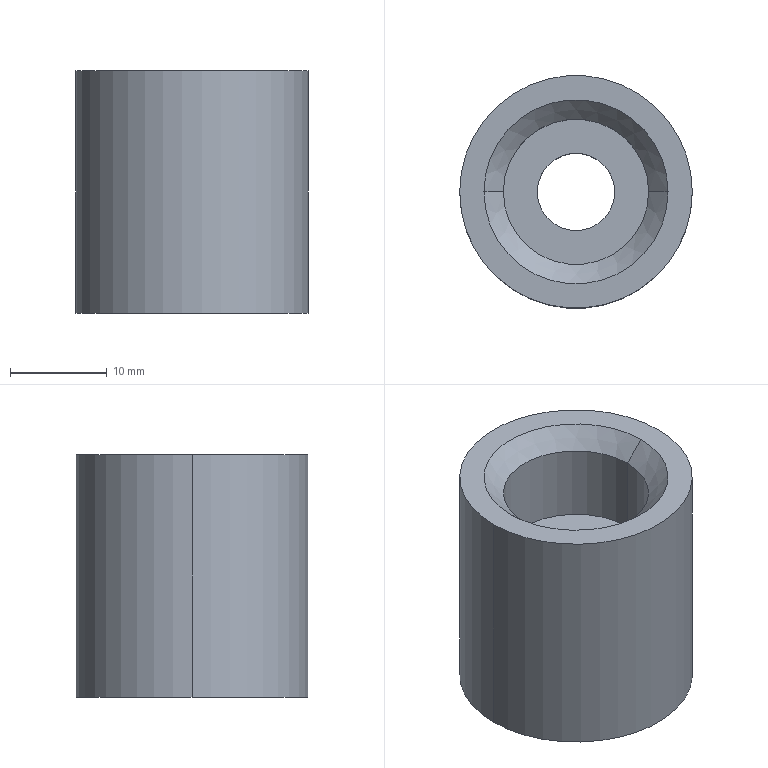Part | STEP file | Elastic block | 1 solid | 13 faces | box 24 x 24 x 25 mm | volume 8627 mm3 | cylinder 6 | cone 4 | plane 3 | commonest cylinder face diameters 8 x2 15 x2 24 x2
STEP:
#1=CARTESIAN_POINT('',(-12.,0.,25.));
#2=VERTEX_POINT('',#1);
#3=CARTESIAN_POINT('',(12.,0.,25.));
#4=VERTEX_POINT('',#3);
#5=CARTESIAN_POINT('',(0.,0.,25.));
#6=DIRECTION('',(0.,0.,-1.));
#7=DIRECTION('',(-1.,0.,0.));
#8=AXIS2_PLACEMENT_3D('',#5,#6,#7);
#9=CIRCLE('',#8,12.);
#10=EDGE_CURVE('',#2,#4,#9,.T.);
#11=ORIENTED_EDGE('',*,*,#10,.T.);
#12=CARTESIAN_POINT('',(12.,0.,0.));
#13=VERTEX_POINT('',#12);
#14=CARTESIAN_POINT('',(12.,0.,25.));
#15=DIRECTION('',(0.,0.,-1.));
#16=VECTOR('',#15,1000.);
#17=LINE('',#14,#16);
#18=EDGE_CURVE('',#4,#13,#17,.T.);
#19=ORIENTED_EDGE('',*,*,#18,.T.);
#20=CARTESIAN_POINT('',(-12.,0.,0.));
#21=VERTEX_POINT('',#20);
#22=CARTESIAN_POINT('',(0.,0.,0.));
#23=DIRECTION('',(0.,0.,1.));
#24=DIRECTION('',(-1.,0.,0.));
#25=AXIS2_PLACEMENT_3D('',#22,#23,#24);
#26=CIRCLE('',#25,12.);
#27=EDGE_CURVE('',#13,#21,#26,.T.);
#28=ORIENTED_EDGE('',*,*,#27,.T.);
#29=CARTESIAN_POINT('',(-12.,0.,25.));
#30=DIRECTION('',(0.,0.,-1.));
#31=VECTOR('',#30,1000.);
#32=LINE('',#29,#31);
#33=EDGE_CURVE('',#2,#21,#32,.T.);
#34=ORIENTED_EDGE('',*,*,#33,.F.);
#35=EDGE_LOOP('',(#11,#19,#28,#34));
#36=FACE_OUTER_BOUND('',#35,.T.);
#37=CARTESIAN_POINT('',(0.,0.,25.));
#38=DIRECTION('',(0.,0.,-1.));
#39=DIRECTION('',(-1.,0.,0.));
#40=AXIS2_PLACEMENT_3D('',#37,#38,#39);
#41=CYLINDRICAL_SURFACE('',#40,12.);
#42=ADVANCED_FACE('',(#36),#41,.T.);
#43=CARTESIAN_POINT('',(4.,0.,2.));
#44=VERTEX_POINT('',#43);
#45=CARTESIAN_POINT('',(-4.,0.,2.));
#46=VERTEX_POINT('',#45);
#47=CARTESIAN_POINT('',(0.,0.,2.));
#48=DIRECTION('',(0.,0.,-1.));
#49=DIRECTION('',(-1.,0.,0.));
#50=AXIS2_PLACEMENT_3D('',#47,#48,#49);
#51=CIRCLE('',#50,4.);
#52=EDGE_CURVE('',#44,#46,#51,.T.);
#53=ORIENTED_EDGE('',*,*,#52,.F.);
#54=CARTESIAN_POINT('',(6.,0.,0.));
#55=VERTEX_POINT('',#54);
#56=CARTESIAN_POINT('',(6.,0.,0.));
#57=DIRECTION('',(0.7071,0.,-0.7071));
#58=VECTOR('',#57,1000.);
#59=LINE('',#56,#58);
#60=EDGE_CURVE('',#44,#55,#59,.T.);
#61=ORIENTED_EDGE('',*,*,#60,.T.);
#62=CARTESIAN_POINT('',(-6.,0.,0.));
#63=VERTEX_POINT('',#62);
#64=CARTESIAN_POINT('',(0.,0.,0.));
#65=DIRECTION('',(0.,0.,-1.));
#66=DIRECTION('',(-1.,0.,0.));
#67=AXIS2_PLACEMENT_3D('',#64,#65,#66);
#68=CIRCLE('',#67,6.);
#69=EDGE_CURVE('',#55,#63,#68,.T.);
#70=ORIENTED_EDGE('',*,*,#69,.T.);
#71=CARTESIAN_POINT('',(-6.,0.,0.));
#72=DIRECTION('',(-0.7071,0.,-0.7071));
#73=VECTOR('',#72,1000.);
#74=LINE('',#71,#73);
#75=EDGE_CURVE('',#46,#63,#74,.T.);
#76=ORIENTED_EDGE('',*,*,#75,.F.);
#77=EDGE_LOOP('',(#53,#61,#70,#76));
#78=FACE_OUTER_BOUND('',#77,.T.);
#79=CARTESIAN_POINT('',(0.,0.,0.));
#80=DIRECTION('',(0.,0.,-1.));
#81=DIRECTION('',(-1.,0.,0.));
#82=AXIS2_PLACEMENT_3D('',#79,#80,#81);
#83=CONICAL_SURFACE('',#82,6.,0.7854);
#84=ADVANCED_FACE('',(#78),#83,.F.);
#85=CARTESIAN_POINT('',(-7.5,0.,23.));
#86=VERTEX_POINT('',#85);
#87=CARTESIAN_POINT('',(7.5,0.,23.));
#88=VERTEX_POINT('',#87);
#89=CARTESIAN_POINT('',(0.,0.,23.));
#90=DIRECTION('',(0.,0.,1.));
#91=DIRECTION('',(1.,0.,0.));
#92=AXIS2_PLACEMENT_3D('',#89,#90,#91);
#93=CIRCLE('',#92,7.5);
#94=EDGE_CURVE('',#86,#88,#93,.T.);
#95=ORIENTED_EDGE('',*,*,#94,.F.);
#96=CARTESIAN_POINT('',(-9.5,0.,25.));
#97=VERTEX_POINT('',#96);
#98=CARTESIAN_POINT('',(-9.5,0.,25.));
#99=DIRECTION('',(-0.7071,0.,0.7071));
#100=VECTOR('',#99,1000.);
#101=LINE('',#98,#100);
#102=EDGE_CURVE('',#86,#97,#101,.T.);
#103=ORIENTED_EDGE('',*,*,#102,.T.);
#104=CARTESIAN_POINT('',(9.5,0.,25.));
#105=VERTEX_POINT('',#104);
#106=CARTESIAN_POINT('',(0.,0.,25.));
#107=DIRECTION('',(0.,0.,-1.));
#108=DIRECTION('',(1.,0.,0.));
#109=AXIS2_PLACEMENT_3D('',#106,#107,#108);
#110=CIRCLE('',#109,9.5);
#111=EDGE_CURVE('',#105,#97,#110,.T.);
#112=ORIENTED_EDGE('',*,*,#111,.F.);
#113=CARTESIAN_POINT('',(9.5,0.,25.));
#114=DIRECTION('',(0.7071,0.,0.7071));
#115=VECTOR('',#114,1000.);
#116=LINE('',#113,#115);
#117=EDGE_CURVE('',#88,#105,#116,.T.);
#118=ORIENTED_EDGE('',*,*,#117,.F.);
#119=EDGE_LOOP('',(#95,#103,#112,#118));
#120=FACE_OUTER_BOUND('',#119,.T.);
#121=CARTESIAN_POINT('',(0.,0.,25.));
#122=DIRECTION('',(0.,0.,1.));
#123=DIRECTION('',(1.,0.,0.));
#124=AXIS2_PLACEMENT_3D('',#121,#122,#123);
#125=CONICAL_SURFACE('',#124,9.5,0.7854);
#126=ADVANCED_FACE('',(#120),#125,.F.);
#127=CARTESIAN_POINT('',(4.,0.,15.));
#128=VERTEX_POINT('',#127);
#129=CARTESIAN_POINT('',(-4.,0.,15.));
#130=VERTEX_POINT('',#129);
#131=CARTESIAN_POINT('',(0.,0.,15.));
#132=DIRECTION('',(0.,0.,-1.));
#133=DIRECTION('',(-1.,0.,0.));
#134=AXIS2_PLACEMENT_3D('',#131,#132,#133);
#135=CIRCLE('',#134,4.);
#136=EDGE_CURVE('',#128,#130,#135,.T.);
#137=ORIENTED_EDGE('',*,*,#136,.F.);
#138=CARTESIAN_POINT('',(4.,0.,25.));
#139=DIRECTION('',(0.,0.,-1.));
#140=VECTOR('',#139,1000.);
#141=LINE('',#138,#140);
#142=EDGE_CURVE('',#128,#44,#141,.T.);
#143=ORIENTED_EDGE('',*,*,#142,.T.);
#144=ORIENTED_EDGE('',*,*,#52,.T.);
#145=CARTESIAN_POINT('',(-4.,0.,25.));
#146=DIRECTION('',(0.,0.,-1.));
#147=VECTOR('',#146,1000.);
#148=LINE('',#145,#147);
#149=EDGE_CURVE('',#130,#46,#148,.T.);
#150=ORIENTED_EDGE('',*,*,#149,.F.);
#151=EDGE_LOOP('',(#137,#143,#144,#150));
#152=FACE_OUTER_BOUND('',#151,.T.);
#153=CARTESIAN_POINT('',(0.,0.,25.));
#154=DIRECTION('',(0.,0.,-1.));
#155=DIRECTION('',(-1.,0.,0.));
#156=AXIS2_PLACEMENT_3D('',#153,#154,#155);
#157=CYLINDRICAL_SURFACE('',#156,4.);
#158=ADVANCED_FACE('',(#152),#157,.F.);
#159=CARTESIAN_POINT('',(-7.5,0.,15.));
#160=VERTEX_POINT('',#159);
#161=CARTESIAN_POINT('',(7.5,0.,15.));
#162=VERTEX_POINT('',#161);
#163=CARTESIAN_POINT('',(0.,0.,15.));
#164=DIRECTION('',(0.,0.,1.));
#165=DIRECTION('',(1.,0.,0.));
#166=AXIS2_PLACEMENT_3D('',#163,#164,#165);
#167=CIRCLE('',#166,7.5);
#168=EDGE_CURVE('',#160,#162,#167,.T.);
#169=ORIENTED_EDGE('',*,*,#168,.F.);
#170=CARTESIAN_POINT('',(-7.5,0.,15.));
#171=DIRECTION('',(0.,0.,1.));
#172=VECTOR('',#171,1000.);
#173=LINE('',#170,#172);
#174=EDGE_CURVE('',#160,#86,#173,.T.);
#175=ORIENTED_EDGE('',*,*,#174,.T.);
#176=ORIENTED_EDGE('',*,*,#94,.T.);
#177=CARTESIAN_POINT('',(7.5,0.,15.));
#178=DIRECTION('',(0.,0.,1.));
#179=VECTOR('',#178,1000.);
#180=LINE('',#177,#179);
#181=EDGE_CURVE('',#162,#88,#180,.T.);
#182=ORIENTED_EDGE('',*,*,#181,.F.);
#183=EDGE_LOOP('',(#169,#175,#176,#182));
#184=FACE_OUTER_BOUND('',#183,.T.);
#185=CARTESIAN_POINT('',(0.,0.,15.));
#186=DIRECTION('',(0.,0.,1.));
#187=DIRECTION('',(1.,0.,0.));
#188=AXIS2_PLACEMENT_3D('',#185,#186,#187);
#189=CYLINDRICAL_SURFACE('',#188,7.5);
#190=ADVANCED_FACE('',(#184),#189,.F.);
#191=ORIENTED_EDGE('',*,*,#18,.F.);
#192=CARTESIAN_POINT('',(0.,0.,25.));
#193=DIRECTION('',(0.,0.,-1.));
#194=DIRECTION('',(-1.,0.,0.));
#195=AXIS2_PLACEMENT_3D('',#192,#193,#194);
#196=CIRCLE('',#195,12.);
#197=EDGE_CURVE('',#4,#2,#196,.T.);
#198=ORIENTED_EDGE('',*,*,#197,.T.);
#199=ORIENTED_EDGE('',*,*,#33,.T.);
#200=CARTESIAN_POINT('',(0.,0.,0.));
#201=DIRECTION('',(0.,0.,1.));
#202=DIRECTION('',(-1.,0.,0.));
#203=AXIS2_PLACEMENT_3D('',#200,#201,#202);
#204=CIRCLE('',#203,12.);
#205=EDGE_CURVE('',#21,#13,#204,.T.);
#206=ORIENTED_EDGE('',*,*,#205,.T.);
#207=EDGE_LOOP('',(#191,#198,#199,#206));
#208=FACE_OUTER_BOUND('',#207,.T.);
#209=CARTESIAN_POINT('',(0.,0.,25.));
#210=DIRECTION('',(0.,0.,-1.));
#211=DIRECTION('',(-1.,0.,0.));
#212=AXIS2_PLACEMENT_3D('',#209,#210,#211);
#213=CYLINDRICAL_SURFACE('',#212,12.);
#214=ADVANCED_FACE('',(#208),#213,.T.);
#215=ORIENTED_EDGE('',*,*,#205,.F.);
#216=ORIENTED_EDGE('',*,*,#27,.F.);
#217=EDGE_LOOP('',(#215,#216));
#218=FACE_OUTER_BOUND('',#217,.T.);
#219=CARTESIAN_POINT('',(0.,0.,0.));
#220=DIRECTION('',(0.,0.,-1.));
#221=DIRECTION('',(-1.,0.,0.));
#222=AXIS2_PLACEMENT_3D('',#219,#220,#221);
#223=CIRCLE('',#222,6.);
#224=EDGE_CURVE('',#63,#55,#223,.T.);
#225=ORIENTED_EDGE('',*,*,#224,.F.);
#226=ORIENTED_EDGE('',*,*,#69,.F.);
#227=EDGE_LOOP('',(#225,#226));
#228=FACE_BOUND('',#227,.T.);
#229=CARTESIAN_POINT('',(0.,0.,0.));
#230=DIRECTION('',(0.,0.,1.));
#231=DIRECTION('',(1.,0.,0.));
#232=AXIS2_PLACEMENT_3D('',#229,#230,#231);
#233=PLANE('',#232);
#234=ADVANCED_FACE('',(#218,#228),#233,.F.);
#235=ORIENTED_EDGE('',*,*,#10,.F.);
#236=ORIENTED_EDGE('',*,*,#197,.F.);
#237=EDGE_LOOP('',(#235,#236));
#238=FACE_OUTER_BOUND('',#237,.T.);
#239=ORIENTED_EDGE('',*,*,#111,.T.);
#240=CARTESIAN_POINT('',(0.,0.,25.));
#241=DIRECTION('',(0.,0.,-1.));
#242=DIRECTION('',(1.,0.,0.));
#243=AXIS2_PLACEMENT_3D('',#240,#241,#242);
#244=CIRCLE('',#243,9.5);
#245=EDGE_CURVE('',#97,#105,#244,.T.);
#246=ORIENTED_EDGE('',*,*,#245,.T.);
#247=EDGE_LOOP('',(#239,#246));
#248=FACE_BOUND('',#247,.T.);
#249=CARTESIAN_POINT('',(0.,0.,25.));
#250=DIRECTION('',(0.,0.,1.));
#251=DIRECTION('',(1.,0.,0.));
#252=AXIS2_PLACEMENT_3D('',#249,#250,#251);
#253=PLANE('',#252);
#254=ADVANCED_FACE('',(#238,#248),#253,.T.);
#255=ORIENTED_EDGE('',*,*,#60,.F.);
#256=CARTESIAN_POINT('',(0.,0.,2.));
#257=DIRECTION('',(0.,0.,-1.));
#258=DIRECTION('',(-1.,0.,0.));
#259=AXIS2_PLACEMENT_3D('',#256,#257,#258);
#260=CIRCLE('',#259,4.);
#261=EDGE_CURVE('',#46,#44,#260,.T.);
#262=ORIENTED_EDGE('',*,*,#261,.F.);
#263=ORIENTED_EDGE('',*,*,#75,.T.);
#264=ORIENTED_EDGE('',*,*,#224,.T.);
#265=EDGE_LOOP('',(#255,#262,#263,#264));
#266=FACE_OUTER_BOUND('',#265,.T.);
#267=CARTESIAN_POINT('',(0.,0.,0.));
#268=DIRECTION('',(0.,0.,-1.));
#269=DIRECTION('',(-1.,0.,0.));
#270=AXIS2_PLACEMENT_3D('',#267,#268,#269);
#271=CONICAL_SURFACE('',#270,6.,0.7854);
#272=ADVANCED_FACE('',(#266),#271,.F.);
#273=ORIENTED_EDGE('',*,*,#102,.F.);
#274=CARTESIAN_POINT('',(0.,0.,23.));
#275=DIRECTION('',(0.,0.,1.));
#276=DIRECTION('',(1.,0.,0.));
#277=AXIS2_PLACEMENT_3D('',#274,#275,#276);
#278=CIRCLE('',#277,7.5);
#279=EDGE_CURVE('',#88,#86,#278,.T.);
#280=ORIENTED_EDGE('',*,*,#279,.F.);
#281=ORIENTED_EDGE('',*,*,#117,.T.);
#282=ORIENTED_EDGE('',*,*,#245,.F.);
#283=EDGE_LOOP('',(#273,#280,#281,#282));
#284=FACE_OUTER_BOUND('',#283,.T.);
#285=CARTESIAN_POINT('',(0.,0.,25.));
#286=DIRECTION('',(0.,0.,1.));
#287=DIRECTION('',(1.,0.,0.));
#288=AXIS2_PLACEMENT_3D('',#285,#286,#287);
#289=CONICAL_SURFACE('',#288,9.5,0.7854);
#290=ADVANCED_FACE('',(#284),#289,.F.);
#291=ORIENTED_EDGE('',*,*,#142,.F.);
#292=CARTESIAN_POINT('',(0.,0.,15.));
#293=DIRECTION('',(0.,0.,-1.));
#294=DIRECTION('',(-1.,0.,0.));
#295=AXIS2_PLACEMENT_3D('',#292,#293,#294);
#296=CIRCLE('',#295,4.);
#297=EDGE_CURVE('',#130,#128,#296,.T.);
#298=ORIENTED_EDGE('',*,*,#297,.F.);
#299=ORIENTED_EDGE('',*,*,#149,.T.);
#300=ORIENTED_EDGE('',*,*,#261,.T.);
#301=EDGE_LOOP('',(#291,#298,#299,#300));
#302=FACE_OUTER_BOUND('',#301,.T.);
#303=CARTESIAN_POINT('',(0.,0.,25.));
#304=DIRECTION('',(0.,0.,-1.));
#305=DIRECTION('',(-1.,0.,0.));
#306=AXIS2_PLACEMENT_3D('',#303,#304,#305);
#307=CYLINDRICAL_SURFACE('',#306,4.);
#308=ADVANCED_FACE('',(#302),#307,.F.);
#309=ORIENTED_EDGE('',*,*,#174,.F.);
#310=CARTESIAN_POINT('',(0.,0.,15.));
#311=DIRECTION('',(0.,0.,1.));
#312=DIRECTION('',(1.,0.,0.));
#313=AXIS2_PLACEMENT_3D('',#310,#311,#312);
#314=CIRCLE('',#313,7.5);
#315=EDGE_CURVE('',#162,#160,#314,.T.);
#316=ORIENTED_EDGE('',*,*,#315,.F.);
#317=ORIENTED_EDGE('',*,*,#181,.T.);
#318=ORIENTED_EDGE('',*,*,#279,.T.);
#319=EDGE_LOOP('',(#309,#316,#317,#318));
#320=FACE_OUTER_BOUND('',#319,.T.);
#321=CARTESIAN_POINT('',(0.,0.,15.));
#322=DIRECTION('',(0.,0.,1.));
#323=DIRECTION('',(1.,0.,0.));
#324=AXIS2_PLACEMENT_3D('',#321,#322,#323);
#325=CYLINDRICAL_SURFACE('',#324,7.5);
#326=ADVANCED_FACE('',(#320),#325,.F.);
#327=ORIENTED_EDGE('',*,*,#315,.T.);
#328=ORIENTED_EDGE('',*,*,#168,.T.);
#329=EDGE_LOOP('',(#327,#328));
#330=FACE_OUTER_BOUND('',#329,.T.);
#331=ORIENTED_EDGE('',*,*,#297,.T.);
#332=ORIENTED_EDGE('',*,*,#136,.T.);
#333=EDGE_LOOP('',(#331,#332));
#334=FACE_BOUND('',#333,.T.);
#335=CARTESIAN_POINT('',(0.,0.,15.));
#336=DIRECTION('',(0.,0.,1.));
#337=DIRECTION('',(1.,0.,0.));
#338=AXIS2_PLACEMENT_3D('',#335,#336,#337);
#339=PLANE('',#338);
#340=ADVANCED_FACE('',(#330,#334),#339,.T.);
#341=CLOSED_SHELL('',(#42,#84,#126,#158,#190,#214,#234,#254,#272,#290,#308,#326,#340));
#342=MANIFOLD_SOLID_BREP('',#341);
#343=CARTESIAN_POINT('',(0.,0.,0.));
#344=DIRECTION('',(0.,0.,1.));
#345=DIRECTION('',(1.,0.,0.));
#346=AXIS2_PLACEMENT_3D('',#343,#344,#345);
#347=(LENGTH_UNIT()NAMED_UNIT(*)SI_UNIT(.MILLI.,.METRE.));
#348=UNCERTAINTY_MEASURE_WITH_UNIT(LENGTH_MEASURE(0.00001),#347,'','');
#349=(NAMED_UNIT(*)PLANE_ANGLE_UNIT()SI_UNIT($,.RADIAN.));
#350=(NAMED_UNIT(*)SI_UNIT($,.STERADIAN.)SOLID_ANGLE_UNIT());
#351=(GEOMETRIC_REPRESENTATION_CONTEXT(3)GLOBAL_UNCERTAINTY_ASSIGNED_CONTEXT((#348))GLOBAL_UNIT_ASSIGNED_CONTEXT((#347,#349,#350))REPRESENTATION_CONTEXT('',''));
#352=ADVANCED_BREP_SHAPE_REPRESENTATION('',(#342,#346),#351);